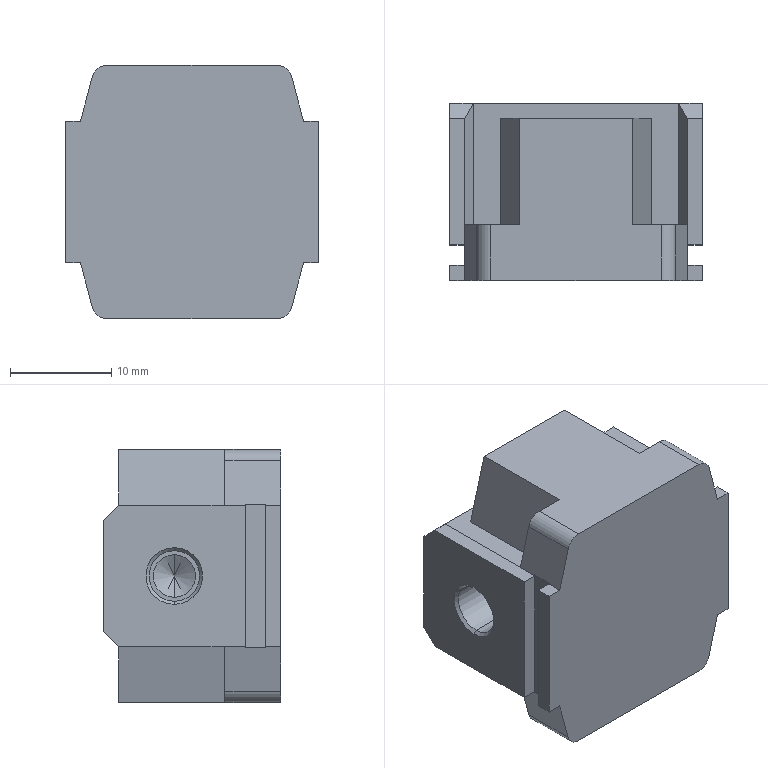Part | STEP file | AC10B-M5_AC3011A AF Body(10)-1 | 1 solid | 72 faces | box 25 x 17.5 x 25 mm | volume 8195 mm3 | plane 52 | cylinder 12 | cone 8 | commonest cylinder face diameters 3 x4 4.2 x4 5 x4